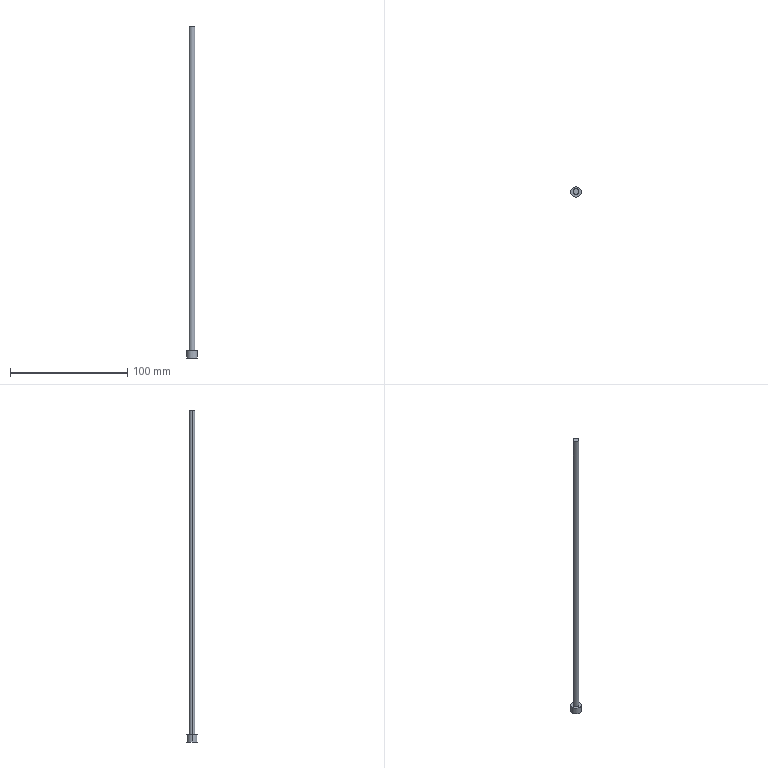Part | Creo | 1 solid | 7 faces | box 9 x 9 x 283.312 mm | volume 5827 mm3 | cylinder 4 | plane 3 | commonest cylinder face diameters 5 x2 9 x2
STEP:
#1=CARTESIAN_POINT('',(-24.5,150.,-12.688));
#2=VERTEX_POINT('',#1);
#3=CARTESIAN_POINT('',(-29.5,150.,-12.688));
#4=VERTEX_POINT('',#3);
#5=CARTESIAN_POINT('',(-27.,150.,-12.688));
#6=DIRECTION('',(0.,0.,1.));
#7=DIRECTION('',(1.,0.,0.));
#8=AXIS2_PLACEMENT_3D('',#5,#6,#7);
#9=CIRCLE('',#8,2.5);
#10=EDGE_CURVE('',#2,#4,#9,.T.);
#11=ORIENTED_EDGE('',*,*,#10,.F.);
#12=CARTESIAN_POINT('',(-27.,150.,-12.688));
#13=DIRECTION('',(0.,0.,1.));
#14=DIRECTION('',(-1.,0.,0.));
#15=AXIS2_PLACEMENT_3D('',#12,#13,#14);
#16=CIRCLE('',#15,2.5);
#17=EDGE_CURVE('',#4,#2,#16,.T.);
#18=ORIENTED_EDGE('',*,*,#17,.F.);
#19=EDGE_LOOP('',(#11,#18));
#20=FACE_OUTER_BOUND('',#19,.F.);
#21=CARTESIAN_POINT('',(0.2984,-1.,-12.688));
#22=DIRECTION('',(0.,0.,1.));
#23=DIRECTION('',(0.,-1.,0.));
#24=AXIS2_PLACEMENT_3D('',#21,#22,#23);
#25=PLANE('',#24);
#26=ADVANCED_FACE('',(#20),#25,.T.);
#27=CARTESIAN_POINT('',(-29.5,150.,-290.));
#28=VERTEX_POINT('',#27);
#29=CARTESIAN_POINT('',(-24.5,150.,-290.));
#30=VERTEX_POINT('',#29);
#31=CARTESIAN_POINT('',(-27.,150.,-290.));
#32=DIRECTION('',(0.,0.,-1.));
#33=DIRECTION('',(-1.,0.,0.));
#34=AXIS2_PLACEMENT_3D('',#31,#32,#33);
#35=CIRCLE('',#34,2.5);
#36=EDGE_CURVE('',#28,#30,#35,.T.);
#37=ORIENTED_EDGE('',*,*,#36,.T.);
#38=CARTESIAN_POINT('',(-24.5,150.,-290.));
#39=DIRECTION('',(0.,0.,1.));
#40=VECTOR('',#39,277.312);
#41=LINE('',#38,#40);
#42=EDGE_CURVE('',#30,#2,#41,.T.);
#43=ORIENTED_EDGE('',*,*,#42,.T.);
#44=ORIENTED_EDGE('',*,*,#10,.T.);
#45=CARTESIAN_POINT('',(-29.5,150.,-290.));
#46=DIRECTION('',(0.,0.,1.));
#47=VECTOR('',#46,277.312);
#48=LINE('',#45,#47);
#49=EDGE_CURVE('',#28,#4,#48,.T.);
#50=ORIENTED_EDGE('',*,*,#49,.F.);
#51=EDGE_LOOP('',(#37,#43,#44,#50));
#52=FACE_OUTER_BOUND('',#51,.F.);
#53=CARTESIAN_POINT('',(-27.,150.,-350.674));
#54=DIRECTION('',(0.,0.,1.));
#55=DIRECTION('',(1.,0.,0.));
#56=AXIS2_PLACEMENT_3D('',#53,#54,#55);
#57=CYLINDRICAL_SURFACE('',#56,2.5);
#58=ADVANCED_FACE('',(#52),#57,.T.);
#59=CARTESIAN_POINT('',(-22.5,150.,-290.));
#60=VERTEX_POINT('',#59);
#61=CARTESIAN_POINT('',(-31.5,150.,-290.));
#62=VERTEX_POINT('',#61);
#63=CARTESIAN_POINT('',(-27.,150.,-290.));
#64=DIRECTION('',(0.,0.,1.));
#65=DIRECTION('',(1.,0.,0.));
#66=AXIS2_PLACEMENT_3D('',#63,#64,#65);
#67=CIRCLE('',#66,4.5);
#68=EDGE_CURVE('',#60,#62,#67,.T.);
#69=ORIENTED_EDGE('',*,*,#68,.F.);
#70=CARTESIAN_POINT('',(-27.,150.,-290.));
#71=DIRECTION('',(0.,0.,1.));
#72=DIRECTION('',(-1.,0.,0.));
#73=AXIS2_PLACEMENT_3D('',#70,#71,#72);
#74=CIRCLE('',#73,4.5);
#75=EDGE_CURVE('',#62,#60,#74,.T.);
#76=ORIENTED_EDGE('',*,*,#75,.F.);
#77=EDGE_LOOP('',(#69,#76));
#78=FACE_OUTER_BOUND('',#77,.F.);
#79=CARTESIAN_POINT('',(-27.,150.,-290.));
#80=DIRECTION('',(0.,0.,-1.));
#81=DIRECTION('',(1.,0.,0.));
#82=AXIS2_PLACEMENT_3D('',#79,#80,#81);
#83=CIRCLE('',#82,2.5);
#84=EDGE_CURVE('',#30,#28,#83,.T.);
#85=ORIENTED_EDGE('',*,*,#84,.F.);
#86=ORIENTED_EDGE('',*,*,#36,.F.);
#87=EDGE_LOOP('',(#85,#86));
#88=FACE_BOUND('',#87,.F.);
#89=CARTESIAN_POINT('',(-27.,150.,-290.));
#90=DIRECTION('',(0.,0.,1.));
#91=DIRECTION('',(-1.,0.,0.));
#92=AXIS2_PLACEMENT_3D('',#89,#90,#91);
#93=PLANE('',#92);
#94=ADVANCED_FACE('',(#78,#88),#93,.T.);
#95=ORIENTED_EDGE('',*,*,#84,.T.);
#96=ORIENTED_EDGE('',*,*,#49,.T.);
#97=ORIENTED_EDGE('',*,*,#17,.T.);
#98=ORIENTED_EDGE('',*,*,#42,.F.);
#99=EDGE_LOOP('',(#95,#96,#97,#98));
#100=FACE_OUTER_BOUND('',#99,.F.);
#101=CARTESIAN_POINT('',(-27.,150.,-350.674));
#102=DIRECTION('',(0.,0.,1.));
#103=DIRECTION('',(1.,0.,0.));
#104=AXIS2_PLACEMENT_3D('',#101,#102,#103);
#105=CYLINDRICAL_SURFACE('',#104,2.5);
#106=ADVANCED_FACE('',(#100),#105,.T.);
#107=ORIENTED_EDGE('',*,*,#68,.T.);
#108=CARTESIAN_POINT('',(-31.5,150.,-296.));
#109=VERTEX_POINT('',#108);
#110=CARTESIAN_POINT('',(-31.5,150.,-296.));
#111=DIRECTION('',(0.,0.,1.));
#112=VECTOR('',#111,6.);
#113=LINE('',#110,#112);
#114=EDGE_CURVE('',#109,#62,#113,.T.);
#115=ORIENTED_EDGE('',*,*,#114,.F.);
#116=CARTESIAN_POINT('',(-22.5,150.,-296.));
#117=VERTEX_POINT('',#116);
#118=CARTESIAN_POINT('',(-27.,150.,-296.));
#119=DIRECTION('',(0.,0.,-1.));
#120=DIRECTION('',(-1.,0.,0.));
#121=AXIS2_PLACEMENT_3D('',#118,#119,#120);
#122=CIRCLE('',#121,4.5);
#123=EDGE_CURVE('',#109,#117,#122,.T.);
#124=ORIENTED_EDGE('',*,*,#123,.T.);
#125=CARTESIAN_POINT('',(-22.5,150.,-296.));
#126=DIRECTION('',(0.,0.,1.));
#127=VECTOR('',#126,6.);
#128=LINE('',#125,#127);
#129=EDGE_CURVE('',#117,#60,#128,.T.);
#130=ORIENTED_EDGE('',*,*,#129,.T.);
#131=EDGE_LOOP('',(#107,#115,#124,#130));
#132=FACE_OUTER_BOUND('',#131,.F.);
#133=CARTESIAN_POINT('',(-27.,150.,-296.));
#134=DIRECTION('',(0.,0.,1.));
#135=DIRECTION('',(-1.,0.,0.));
#136=AXIS2_PLACEMENT_3D('',#133,#134,#135);
#137=CYLINDRICAL_SURFACE('',#136,4.5);
#138=ADVANCED_FACE('',(#132),#137,.T.);
#139=ORIENTED_EDGE('',*,*,#75,.T.);
#140=ORIENTED_EDGE('',*,*,#129,.F.);
#141=CARTESIAN_POINT('',(-27.,150.,-296.));
#142=DIRECTION('',(0.,0.,-1.));
#143=DIRECTION('',(1.,0.,0.));
#144=AXIS2_PLACEMENT_3D('',#141,#142,#143);
#145=CIRCLE('',#144,4.5);
#146=EDGE_CURVE('',#117,#109,#145,.T.);
#147=ORIENTED_EDGE('',*,*,#146,.T.);
#148=ORIENTED_EDGE('',*,*,#114,.T.);
#149=EDGE_LOOP('',(#139,#140,#147,#148));
#150=FACE_OUTER_BOUND('',#149,.F.);
#151=CARTESIAN_POINT('',(-27.,150.,-296.));
#152=DIRECTION('',(0.,0.,1.));
#153=DIRECTION('',(-1.,0.,0.));
#154=AXIS2_PLACEMENT_3D('',#151,#152,#153);
#155=CYLINDRICAL_SURFACE('',#154,4.5);
#156=ADVANCED_FACE('',(#150),#155,.T.);
#157=ORIENTED_EDGE('',*,*,#146,.F.);
#158=ORIENTED_EDGE('',*,*,#123,.F.);
#159=EDGE_LOOP('',(#157,#158));
#160=FACE_OUTER_BOUND('',#159,.F.);
#161=CARTESIAN_POINT('',(10.298,-0.9953,-296.));
#162=DIRECTION('',(0.,0.,1.));
#163=DIRECTION('',(0.,-1.,0.));
#164=AXIS2_PLACEMENT_3D('',#161,#162,#163);
#165=PLANE('',#164);
#166=ADVANCED_FACE('',(#160),#165,.F.);
#167=CLOSED_SHELL('',(#26,#58,#94,#106,#138,#156,#166));
#168=MANIFOLD_SOLID_BREP('',#167);
#169=(LENGTH_UNIT()NAMED_UNIT(*)SI_UNIT(.MILLI.,.METRE.));
#170=UNCERTAINTY_MEASURE_WITH_UNIT(LENGTH_MEASURE(0.02836),#169,'','');
#171=(NAMED_UNIT(*)PLANE_ANGLE_UNIT()SI_UNIT($,.RADIAN.));
#172=PLANE_ANGLE_MEASURE_WITH_UNIT(PLANE_ANGLE_MEASURE(0.01745),#171);
#173=(CONVERSION_BASED_UNIT('DEGREE',#172)NAMED_UNIT(*)PLANE_ANGLE_UNIT());
#174=(NAMED_UNIT(*)SI_UNIT($,.STERADIAN.)SOLID_ANGLE_UNIT());
#175=(GEOMETRIC_REPRESENTATION_CONTEXT(3)GLOBAL_UNCERTAINTY_ASSIGNED_CONTEXT((#170))GLOBAL_UNIT_ASSIGNED_CONTEXT((#169,#173,#174))REPRESENTATION_CONTEXT('',''));
#176=ADVANCED_BREP_SHAPE_REPRESENTATION('',(#168),#175);